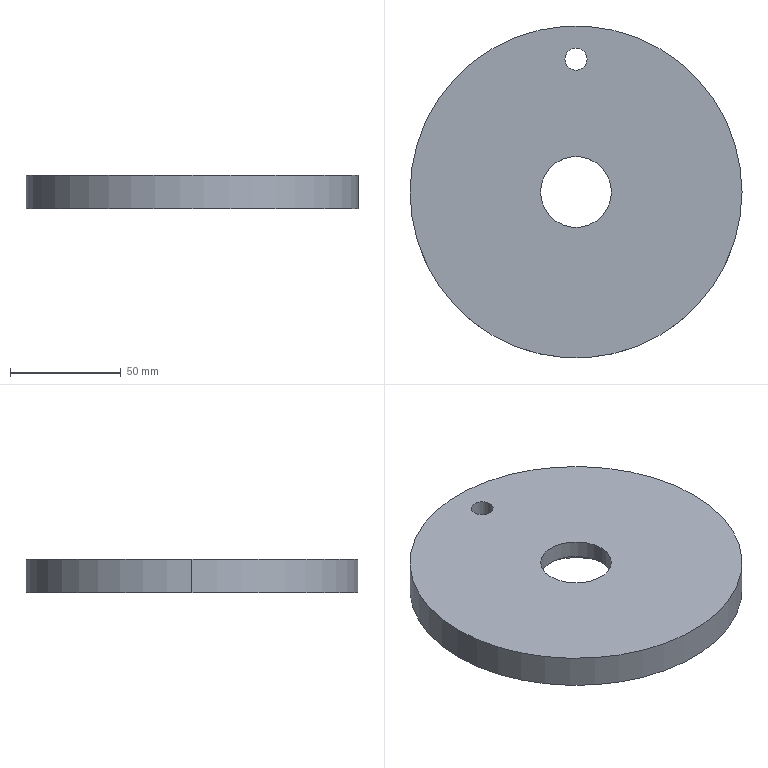Part | SolidWorks | features Extrusion 1, ICE 1 | 1 solid | 11 faces | box 150 x 150 x 15 mm | volume 243715 mm3 | cylinder 8 | plane 3 | commonest cylinder face diameters 10 x2 32 x2 50 x2 150 x2
STEP:
#1=CARTESIAN_POINT('',(-25.,0.,7.));
#2=VERTEX_POINT('',#1);
#3=CARTESIAN_POINT('',(25.,0.,7.));
#4=VERTEX_POINT('',#3);
#5=CARTESIAN_POINT('',(0.,0.,7.));
#6=DIRECTION('',(0.,0.,1.));
#7=DIRECTION('',(1.,0.,0.));
#8=AXIS2_PLACEMENT_3D('',#5,#6,#7);
#9=CIRCLE('',#8,25.);
#10=EDGE_CURVE('',#2,#4,#9,.T.);
#11=ORIENTED_EDGE('',*,*,#10,.T.);
#12=CARTESIAN_POINT('',(25.,0.,0.));
#13=VERTEX_POINT('',#12);
#14=CARTESIAN_POINT('',(25.,0.,7.));
#15=DIRECTION('',(0.,0.,-1.));
#16=VECTOR('',#15,1000.);
#17=LINE('',#14,#16);
#18=EDGE_CURVE('',#4,#13,#17,.T.);
#19=ORIENTED_EDGE('',*,*,#18,.T.);
#20=CARTESIAN_POINT('',(-25.,0.,0.));
#21=VERTEX_POINT('',#20);
#22=CARTESIAN_POINT('',(0.,0.,0.));
#23=DIRECTION('',(0.,0.,1.));
#24=DIRECTION('',(1.,0.,0.));
#25=AXIS2_PLACEMENT_3D('',#22,#23,#24);
#26=CIRCLE('',#25,25.);
#27=EDGE_CURVE('',#21,#13,#26,.T.);
#28=ORIENTED_EDGE('',*,*,#27,.F.);
#29=CARTESIAN_POINT('',(-25.,0.,7.));
#30=DIRECTION('',(0.,0.,-1.));
#31=VECTOR('',#30,1000.);
#32=LINE('',#29,#31);
#33=EDGE_CURVE('',#2,#21,#32,.T.);
#34=ORIENTED_EDGE('',*,*,#33,.F.);
#35=EDGE_LOOP('',(#11,#19,#28,#34));
#36=FACE_OUTER_BOUND('',#35,.T.);
#37=CARTESIAN_POINT('',(0.,0.,7.));
#38=DIRECTION('',(0.,0.,-1.));
#39=DIRECTION('',(-1.,0.,0.));
#40=AXIS2_PLACEMENT_3D('',#37,#38,#39);
#41=CYLINDRICAL_SURFACE('',#40,25.);
#42=ADVANCED_FACE('',(#36),#41,.F.);
#43=CARTESIAN_POINT('',(-16.,0.,15.));
#44=VERTEX_POINT('',#43);
#45=CARTESIAN_POINT('',(16.,0.,15.));
#46=VERTEX_POINT('',#45);
#47=CARTESIAN_POINT('',(0.,0.,15.));
#48=DIRECTION('',(0.,0.,1.));
#49=DIRECTION('',(1.,0.,0.));
#50=AXIS2_PLACEMENT_3D('',#47,#48,#49);
#51=CIRCLE('',#50,16.);
#52=EDGE_CURVE('',#44,#46,#51,.T.);
#53=ORIENTED_EDGE('',*,*,#52,.T.);
#54=CARTESIAN_POINT('',(16.,0.,7.));
#55=VERTEX_POINT('',#54);
#56=CARTESIAN_POINT('',(16.,0.,15.));
#57=DIRECTION('',(0.,0.,-1.));
#58=VECTOR('',#57,1000.);
#59=LINE('',#56,#58);
#60=EDGE_CURVE('',#46,#55,#59,.T.);
#61=ORIENTED_EDGE('',*,*,#60,.T.);
#62=CARTESIAN_POINT('',(-16.,0.,7.));
#63=VERTEX_POINT('',#62);
#64=CARTESIAN_POINT('',(0.,0.,7.));
#65=DIRECTION('',(0.,0.,1.));
#66=DIRECTION('',(1.,0.,0.));
#67=AXIS2_PLACEMENT_3D('',#64,#65,#66);
#68=CIRCLE('',#67,16.);
#69=EDGE_CURVE('',#63,#55,#68,.T.);
#70=ORIENTED_EDGE('',*,*,#69,.F.);
#71=CARTESIAN_POINT('',(-16.,0.,15.));
#72=DIRECTION('',(0.,0.,-1.));
#73=VECTOR('',#72,1000.);
#74=LINE('',#71,#73);
#75=EDGE_CURVE('',#44,#63,#74,.T.);
#76=ORIENTED_EDGE('',*,*,#75,.F.);
#77=EDGE_LOOP('',(#53,#61,#70,#76));
#78=FACE_OUTER_BOUND('',#77,.T.);
#79=CARTESIAN_POINT('',(0.,0.,15.));
#80=DIRECTION('',(0.,0.,-1.));
#81=DIRECTION('',(-1.,0.,0.));
#82=AXIS2_PLACEMENT_3D('',#79,#80,#81);
#83=CYLINDRICAL_SURFACE('',#82,16.);
#84=ADVANCED_FACE('',(#78),#83,.F.);
#85=CARTESIAN_POINT('',(-5.,60.,15.));
#86=VERTEX_POINT('',#85);
#87=CARTESIAN_POINT('',(5.,60.,15.));
#88=VERTEX_POINT('',#87);
#89=CARTESIAN_POINT('',(0.,60.,15.));
#90=DIRECTION('',(0.,0.,1.));
#91=DIRECTION('',(1.,0.,0.));
#92=AXIS2_PLACEMENT_3D('',#89,#90,#91);
#93=CIRCLE('',#92,5.);
#94=EDGE_CURVE('',#86,#88,#93,.T.);
#95=ORIENTED_EDGE('',*,*,#94,.T.);
#96=CARTESIAN_POINT('',(5.,60.,0.));
#97=VERTEX_POINT('',#96);
#98=CARTESIAN_POINT('',(5.,60.,15.));
#99=DIRECTION('',(0.,0.,-1.));
#100=VECTOR('',#99,1000.);
#101=LINE('',#98,#100);
#102=EDGE_CURVE('',#88,#97,#101,.T.);
#103=ORIENTED_EDGE('',*,*,#102,.T.);
#104=CARTESIAN_POINT('',(-5.,60.,0.));
#105=VERTEX_POINT('',#104);
#106=CARTESIAN_POINT('',(0.,60.,0.));
#107=DIRECTION('',(0.,0.,1.));
#108=DIRECTION('',(1.,0.,0.));
#109=AXIS2_PLACEMENT_3D('',#106,#107,#108);
#110=CIRCLE('',#109,5.);
#111=EDGE_CURVE('',#105,#97,#110,.T.);
#112=ORIENTED_EDGE('',*,*,#111,.F.);
#113=CARTESIAN_POINT('',(-5.,60.,15.));
#114=DIRECTION('',(0.,0.,-1.));
#115=VECTOR('',#114,1000.);
#116=LINE('',#113,#115);
#117=EDGE_CURVE('',#86,#105,#116,.T.);
#118=ORIENTED_EDGE('',*,*,#117,.F.);
#119=EDGE_LOOP('',(#95,#103,#112,#118));
#120=FACE_OUTER_BOUND('',#119,.T.);
#121=CARTESIAN_POINT('',(0.,60.,15.));
#122=DIRECTION('',(0.,0.,-1.));
#123=DIRECTION('',(-1.,0.,0.));
#124=AXIS2_PLACEMENT_3D('',#121,#122,#123);
#125=CYLINDRICAL_SURFACE('',#124,5.);
#126=ADVANCED_FACE('',(#120),#125,.F.);
#127=CARTESIAN_POINT('',(75.,0.,15.));
#128=VERTEX_POINT('',#127);
#129=CARTESIAN_POINT('',(-75.,0.,15.));
#130=VERTEX_POINT('',#129);
#131=CARTESIAN_POINT('',(0.,0.,15.));
#132=DIRECTION('',(0.,0.,1.));
#133=DIRECTION('',(1.,0.,0.));
#134=AXIS2_PLACEMENT_3D('',#131,#132,#133);
#135=CIRCLE('',#134,75.);
#136=EDGE_CURVE('',#128,#130,#135,.T.);
#137=ORIENTED_EDGE('',*,*,#136,.F.);
#138=CARTESIAN_POINT('',(75.,0.,0.));
#139=VERTEX_POINT('',#138);
#140=CARTESIAN_POINT('',(75.,0.,15.));
#141=DIRECTION('',(0.,0.,-1.));
#142=VECTOR('',#141,1000.);
#143=LINE('',#140,#142);
#144=EDGE_CURVE('',#128,#139,#143,.T.);
#145=ORIENTED_EDGE('',*,*,#144,.T.);
#146=CARTESIAN_POINT('',(-75.,0.,0.));
#147=VERTEX_POINT('',#146);
#148=CARTESIAN_POINT('',(0.,0.,0.));
#149=DIRECTION('',(0.,0.,1.));
#150=DIRECTION('',(1.,0.,0.));
#151=AXIS2_PLACEMENT_3D('',#148,#149,#150);
#152=CIRCLE('',#151,75.);
#153=EDGE_CURVE('',#139,#147,#152,.T.);
#154=ORIENTED_EDGE('',*,*,#153,.T.);
#155=CARTESIAN_POINT('',(-75.,0.,15.));
#156=DIRECTION('',(0.,0.,-1.));
#157=VECTOR('',#156,1000.);
#158=LINE('',#155,#157);
#159=EDGE_CURVE('',#130,#147,#158,.T.);
#160=ORIENTED_EDGE('',*,*,#159,.F.);
#161=EDGE_LOOP('',(#137,#145,#154,#160));
#162=FACE_OUTER_BOUND('',#161,.T.);
#163=CARTESIAN_POINT('',(0.,0.,15.));
#164=DIRECTION('',(0.,0.,-1.));
#165=DIRECTION('',(-1.,0.,0.));
#166=AXIS2_PLACEMENT_3D('',#163,#164,#165);
#167=CYLINDRICAL_SURFACE('',#166,75.);
#168=ADVANCED_FACE('',(#162),#167,.T.);
#169=ORIENTED_EDGE('',*,*,#94,.F.);
#170=CARTESIAN_POINT('',(0.,60.,15.));
#171=DIRECTION('',(0.,0.,1.));
#172=DIRECTION('',(1.,0.,0.));
#173=AXIS2_PLACEMENT_3D('',#170,#171,#172);
#174=CIRCLE('',#173,5.);
#175=EDGE_CURVE('',#88,#86,#174,.T.);
#176=ORIENTED_EDGE('',*,*,#175,.F.);
#177=EDGE_LOOP('',(#169,#176));
#178=FACE_BOUND('',#177,.T.);
#179=CARTESIAN_POINT('',(0.,0.,15.));
#180=DIRECTION('',(0.,0.,1.));
#181=DIRECTION('',(1.,0.,0.));
#182=AXIS2_PLACEMENT_3D('',#179,#180,#181);
#183=CIRCLE('',#182,75.);
#184=EDGE_CURVE('',#130,#128,#183,.T.);
#185=ORIENTED_EDGE('',*,*,#184,.T.);
#186=ORIENTED_EDGE('',*,*,#136,.T.);
#187=EDGE_LOOP('',(#185,#186));
#188=FACE_OUTER_BOUND('',#187,.T.);
#189=ORIENTED_EDGE('',*,*,#52,.F.);
#190=CARTESIAN_POINT('',(0.,0.,15.));
#191=DIRECTION('',(0.,0.,1.));
#192=DIRECTION('',(1.,0.,0.));
#193=AXIS2_PLACEMENT_3D('',#190,#191,#192);
#194=CIRCLE('',#193,16.);
#195=EDGE_CURVE('',#46,#44,#194,.T.);
#196=ORIENTED_EDGE('',*,*,#195,.F.);
#197=EDGE_LOOP('',(#189,#196));
#198=FACE_BOUND('',#197,.T.);
#199=CARTESIAN_POINT('',(0.,0.,15.));
#200=DIRECTION('',(0.,0.,1.));
#201=DIRECTION('',(1.,0.,0.));
#202=AXIS2_PLACEMENT_3D('',#199,#200,#201);
#203=PLANE('',#202);
#204=ADVANCED_FACE('',(#178,#188,#198),#203,.T.);
#205=ORIENTED_EDGE('',*,*,#27,.T.);
#206=CARTESIAN_POINT('',(0.,0.,0.));
#207=DIRECTION('',(0.,0.,1.));
#208=DIRECTION('',(1.,0.,0.));
#209=AXIS2_PLACEMENT_3D('',#206,#207,#208);
#210=CIRCLE('',#209,25.);
#211=EDGE_CURVE('',#13,#21,#210,.T.);
#212=ORIENTED_EDGE('',*,*,#211,.T.);
#213=EDGE_LOOP('',(#205,#212));
#214=FACE_BOUND('',#213,.T.);
#215=CARTESIAN_POINT('',(0.,0.,0.));
#216=DIRECTION('',(0.,0.,1.));
#217=DIRECTION('',(1.,0.,0.));
#218=AXIS2_PLACEMENT_3D('',#215,#216,#217);
#219=CIRCLE('',#218,75.);
#220=EDGE_CURVE('',#147,#139,#219,.T.);
#221=ORIENTED_EDGE('',*,*,#220,.F.);
#222=ORIENTED_EDGE('',*,*,#153,.F.);
#223=EDGE_LOOP('',(#221,#222));
#224=FACE_OUTER_BOUND('',#223,.T.);
#225=ORIENTED_EDGE('',*,*,#111,.T.);
#226=CARTESIAN_POINT('',(0.,60.,0.));
#227=DIRECTION('',(0.,0.,1.));
#228=DIRECTION('',(1.,0.,0.));
#229=AXIS2_PLACEMENT_3D('',#226,#227,#228);
#230=CIRCLE('',#229,5.);
#231=EDGE_CURVE('',#97,#105,#230,.T.);
#232=ORIENTED_EDGE('',*,*,#231,.T.);
#233=EDGE_LOOP('',(#225,#232));
#234=FACE_BOUND('',#233,.T.);
#235=CARTESIAN_POINT('',(0.,0.,0.));
#236=DIRECTION('',(0.,0.,1.));
#237=DIRECTION('',(1.,0.,0.));
#238=AXIS2_PLACEMENT_3D('',#235,#236,#237);
#239=PLANE('',#238);
#240=ADVANCED_FACE('',(#214,#224,#234),#239,.F.);
#241=ORIENTED_EDGE('',*,*,#144,.F.);
#242=ORIENTED_EDGE('',*,*,#184,.F.);
#243=ORIENTED_EDGE('',*,*,#159,.T.);
#244=ORIENTED_EDGE('',*,*,#220,.T.);
#245=EDGE_LOOP('',(#241,#242,#243,#244));
#246=FACE_OUTER_BOUND('',#245,.T.);
#247=CARTESIAN_POINT('',(0.,0.,15.));
#248=DIRECTION('',(0.,0.,-1.));
#249=DIRECTION('',(-1.,0.,0.));
#250=AXIS2_PLACEMENT_3D('',#247,#248,#249);
#251=CYLINDRICAL_SURFACE('',#250,75.);
#252=ADVANCED_FACE('',(#246),#251,.T.);
#253=ORIENTED_EDGE('',*,*,#102,.F.);
#254=ORIENTED_EDGE('',*,*,#175,.T.);
#255=ORIENTED_EDGE('',*,*,#117,.T.);
#256=ORIENTED_EDGE('',*,*,#231,.F.);
#257=EDGE_LOOP('',(#253,#254,#255,#256));
#258=FACE_OUTER_BOUND('',#257,.T.);
#259=CARTESIAN_POINT('',(0.,60.,15.));
#260=DIRECTION('',(0.,0.,-1.));
#261=DIRECTION('',(-1.,0.,0.));
#262=AXIS2_PLACEMENT_3D('',#259,#260,#261);
#263=CYLINDRICAL_SURFACE('',#262,5.);
#264=ADVANCED_FACE('',(#258),#263,.F.);
#265=ORIENTED_EDGE('',*,*,#60,.F.);
#266=ORIENTED_EDGE('',*,*,#195,.T.);
#267=ORIENTED_EDGE('',*,*,#75,.T.);
#268=CARTESIAN_POINT('',(0.,0.,7.));
#269=DIRECTION('',(0.,0.,1.));
#270=DIRECTION('',(1.,0.,0.));
#271=AXIS2_PLACEMENT_3D('',#268,#269,#270);
#272=CIRCLE('',#271,16.);
#273=EDGE_CURVE('',#55,#63,#272,.T.);
#274=ORIENTED_EDGE('',*,*,#273,.F.);
#275=EDGE_LOOP('',(#265,#266,#267,#274));
#276=FACE_OUTER_BOUND('',#275,.T.);
#277=CARTESIAN_POINT('',(0.,0.,15.));
#278=DIRECTION('',(0.,0.,-1.));
#279=DIRECTION('',(-1.,0.,0.));
#280=AXIS2_PLACEMENT_3D('',#277,#278,#279);
#281=CYLINDRICAL_SURFACE('',#280,16.);
#282=ADVANCED_FACE('',(#276),#281,.F.);
#283=ORIENTED_EDGE('',*,*,#18,.F.);
#284=CARTESIAN_POINT('',(0.,0.,7.));
#285=DIRECTION('',(0.,0.,1.));
#286=DIRECTION('',(1.,0.,0.));
#287=AXIS2_PLACEMENT_3D('',#284,#285,#286);
#288=CIRCLE('',#287,25.);
#289=EDGE_CURVE('',#4,#2,#288,.T.);
#290=ORIENTED_EDGE('',*,*,#289,.T.);
#291=ORIENTED_EDGE('',*,*,#33,.T.);
#292=ORIENTED_EDGE('',*,*,#211,.F.);
#293=EDGE_LOOP('',(#283,#290,#291,#292));
#294=FACE_OUTER_BOUND('',#293,.T.);
#295=CARTESIAN_POINT('',(0.,0.,7.));
#296=DIRECTION('',(0.,0.,-1.));
#297=DIRECTION('',(-1.,0.,0.));
#298=AXIS2_PLACEMENT_3D('',#295,#296,#297);
#299=CYLINDRICAL_SURFACE('',#298,25.);
#300=ADVANCED_FACE('',(#294),#299,.F.);
#301=ORIENTED_EDGE('',*,*,#69,.T.);
#302=ORIENTED_EDGE('',*,*,#273,.T.);
#303=EDGE_LOOP('',(#301,#302));
#304=FACE_BOUND('',#303,.T.);
#305=ORIENTED_EDGE('',*,*,#10,.F.);
#306=ORIENTED_EDGE('',*,*,#289,.F.);
#307=EDGE_LOOP('',(#305,#306));
#308=FACE_OUTER_BOUND('',#307,.T.);
#309=CARTESIAN_POINT('',(0.,0.,7.));
#310=DIRECTION('',(0.,0.,1.));
#311=DIRECTION('',(1.,0.,0.));
#312=AXIS2_PLACEMENT_3D('',#309,#310,#311);
#313=PLANE('',#312);
#314=ADVANCED_FACE('',(#304,#308),#313,.F.);
#315=CLOSED_SHELL('',(#42,#84,#126,#168,#204,#240,#252,#264,#282,#300,#314));
#316=MANIFOLD_SOLID_BREP('',#315);
#317=CARTESIAN_POINT('',(0.,0.,0.));
#318=DIRECTION('',(0.,0.,1.));
#319=DIRECTION('',(1.,0.,0.));
#320=AXIS2_PLACEMENT_3D('',#317,#318,#319);
#321=(LENGTH_UNIT()NAMED_UNIT(*)SI_UNIT(.MILLI.,.METRE.));
#322=UNCERTAINTY_MEASURE_WITH_UNIT(LENGTH_MEASURE(0.00001),#321,'','');
#323=(NAMED_UNIT(*)PLANE_ANGLE_UNIT()SI_UNIT($,.RADIAN.));
#324=(NAMED_UNIT(*)SI_UNIT($,.STERADIAN.)SOLID_ANGLE_UNIT());
#325=(GEOMETRIC_REPRESENTATION_CONTEXT(3)GLOBAL_UNCERTAINTY_ASSIGNED_CONTEXT((#322))GLOBAL_UNIT_ASSIGNED_CONTEXT((#321,#323,#324))REPRESENTATION_CONTEXT('',''));
#326=ADVANCED_BREP_SHAPE_REPRESENTATION('',(#316,#320),#325);